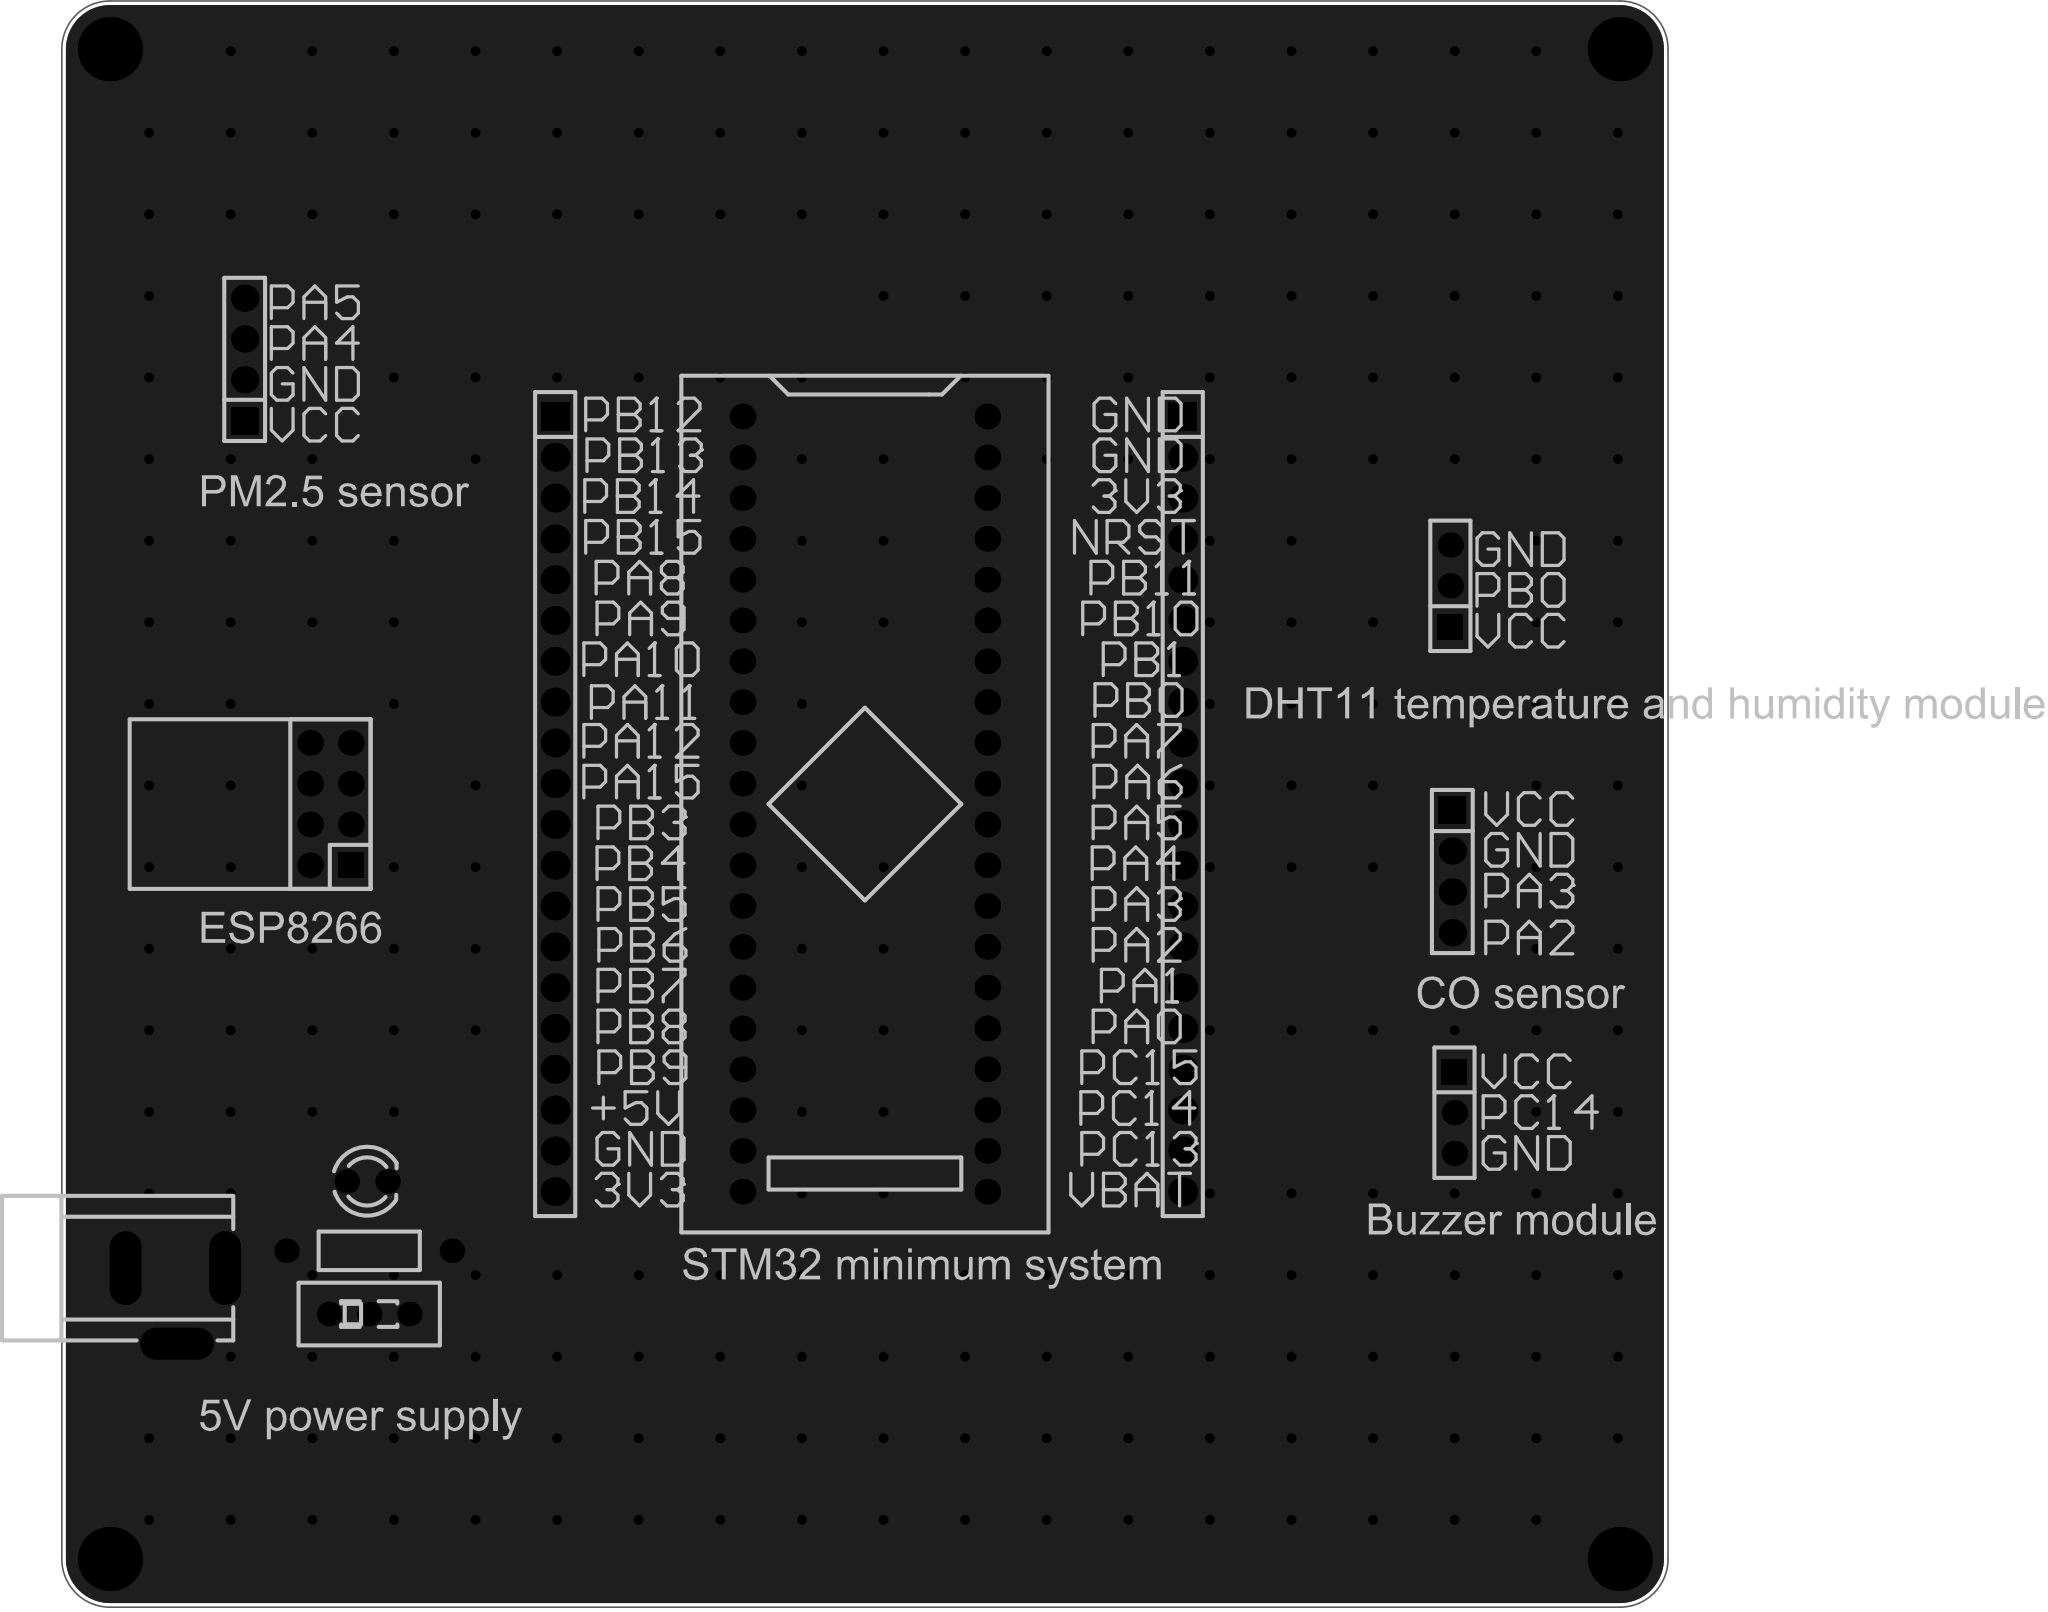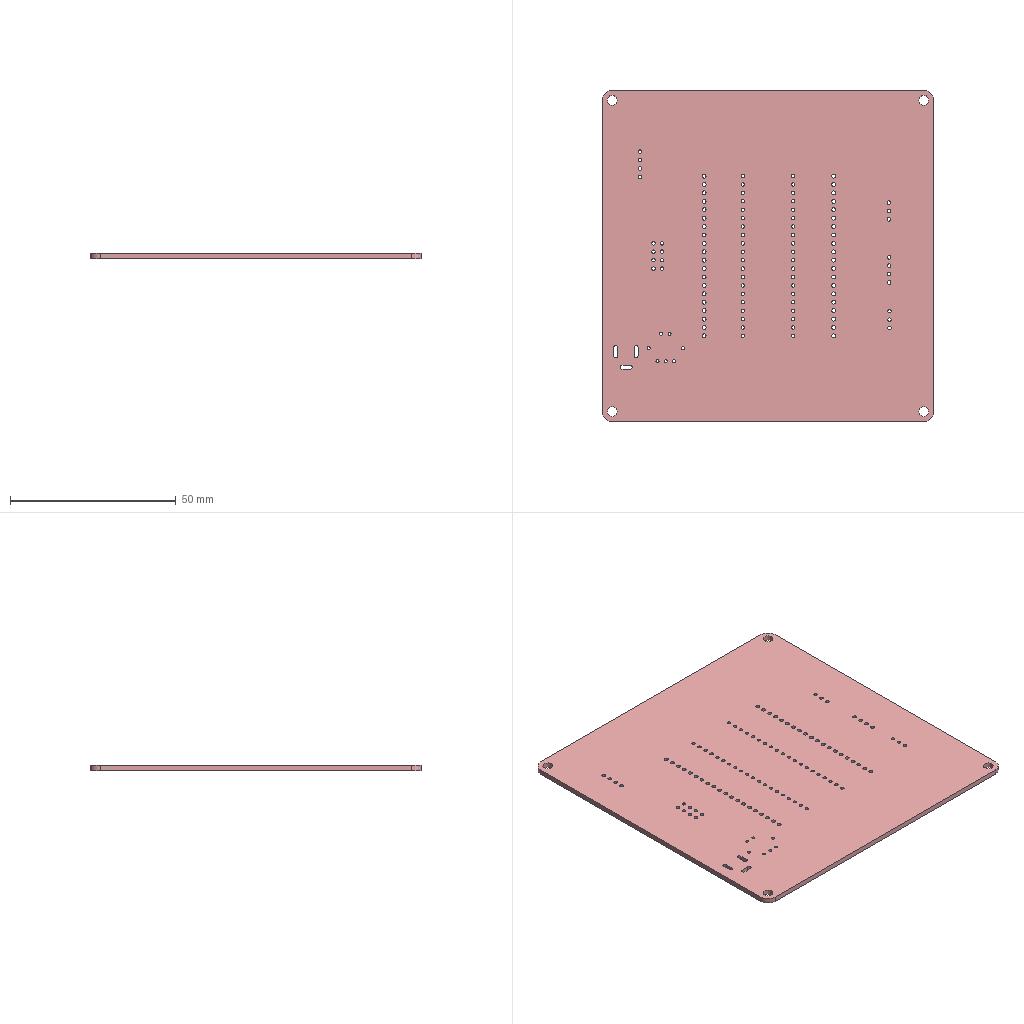Circuit board layout | Altium Designer | box 100 x 100 x 1.6 mm
Layer stack:
# Altium Designer layer stack of  (unit mm; dielectric type: 0 none, 1 core, 2 prepreg, 3 surface material)
index,name,kind,layer,copper_thickness_mm,dielectric_type,dielectric_thickness_mm,dielectric_material,dielectric_constant
0,Top Paste Mask Layer,other,,,,,,
1,Top Silkscreen Layer,other,,,,,,
2,Top Solder Mask Layer,dielectric,,,3,0.01,,3.3
3,Top Layer,copper,Top Layer,0.035,,,,
4,Dielectric1,dielectric,,,3,1.51,FR4,4.5
5,Bottom Layer,copper,Bottom Layer,0.035,,,,
6,Bottom Solder Mask Layer,dielectric,,,3,0.01,,3.3
7,Bottom Silkscreen Layer,other,,,,,,
8,Bottom Paste Mask Layer,other,,,,,,
# drill layer pairs: low layer,high layer
drill_pair,Top Layer,Bottom Layer
Part placement:
Designator,Comment,Layer,Footprint,Center-X(mm),Center-Y(mm),Rotation
U1,STM32F103C8T6-Card,TopLayer,CONN-TH_L53.3-W22.9_STM32F103C8T6-CARD,130.556,128.905,270
DC1,DC005,TopLayer,DC-IN-TH_DC005,87.63,97.663,0
H23,,TopLayer,HDR-TH_4P-P2.54-V-M,167.125,124.707,270
H24,,TopLayer,HDR-TH_4P-P2.54-V-M,91.941,156.591,90
H15,,TopLayer,HDR-TH_3P-P2.54-V-F,167.005,142.494,90
H16,,TopLayer,HDR-TH_8P-P2.54-V-F-R2-C4-S2.54-1,97.282,128.905,90
H1,,TopLayer,HDR-TH_20P-P2.54-V-F,111.273,128.905,270
H2,,TopLayer,HDR-TH_20P-P2.54-V-F,150.344,128.905,270
H18,,TopLayer,HDR-TH_3P-P2.54-V-F,167.259,109.692,270
LED1,,TopLayer,LED_TH-3mm,99.568,105.41,0
R1,330,TopLayer,Res_1/4W,99.695,101.092,180
SW1,Switch,TopLayer,SW-TH_SS-12D01-GX,99.695,97.155,0
Pad and via stacks:
# Altium Designer via and pad stacks of  (unit mm). Each distinct definition once, with the count of objects using it.
# via: kind,start_layer,end_layer,hole_mm,diameter_mm,mode(0 simple;1 top-mid-bottom;2 full stack),diameter_per_layer,count,example_net
# pad: kind,layer,hole_mm,hole_type(0 round;1 square;2 slot),plating,top_size,top_shape(1 round;2 rect;3 octagon;9 rounded rect),mid_size,bottom_size,mode,footprint,size_per_layer,count,example
pad,Multi-Layer,3,0,plated,4x4,1,4x4,4x4,0,,,4,1
pad,Multi-Layer,1,0,plated,1.6x1.6,1,1.6x1.6,1.6x1.6,0,CONN-TH_L53.3-W22.9_STM32F103C8T6-CARD,,40,U1.1
pad,Multi-Layer,1.2,2,plated,2x4.6,1,2x4.6,2x4.6,0,DC-IN-TH_DC005,,2,DC1.1
pad,Multi-Layer,1.2,2,plated,4.6x2,1,4.6x2,4.6x2,0,DC-IN-TH_DC005,,1,DC1.3
pad,Multi-Layer,1.1,0,plated,1.7x1.7,2,1.7x1.7,1.7x1.7,0,HDR-TH_4P-P2.54-V-M,,2,H23.1
pad,Multi-Layer,1.1,0,plated,1.7x1.7,1,1.7x1.7,1.7x1.7,0,HDR-TH_4P-P2.54-V-M,,6,H23.2
pad,Multi-Layer,1.02,0,plated,1.575x1.575,1,1.575x1.575,1.575x1.575,0,HDR-TH_3P-P2.54-V-F,,4,H15.3
pad,Multi-Layer,1.02,0,plated,1.575x1.575,2,1.575x1.575,1.575x1.575,0,HDR-TH_3P-P2.54-V-F,,2,H15.1
pad,Multi-Layer,1.1,0,plated,1.6x1.6,2,1.6x1.6,1.6x1.6,0,HDR-TH_8P-P2.54-V-F-R2-C4-S2.54-1,,1,H16.1
pad,Multi-Layer,1.1,0,plated,1.6x1.6,1,1.6x1.6,1.6x1.6,0,HDR-TH_8P-P2.54-V-F-R2-C4-S2.54-1,,7,H16.2
pad,Multi-Layer,1.2,0,plated,1.8x1.8,2,1.8x1.8,1.8x1.8,0,HDR-TH_20P-P2.54-V-F,,2,H1.1
pad,Multi-Layer,1.2,0,plated,1.8x1.8,1,1.8x1.8,1.8x1.8,0,HDR-TH_20P-P2.54-V-F,,38,H1.2
pad,Multi-Layer,0.9144,0,plated,1.524x1.524,1,1.524x1.524,1.524x1.524,0,LED_TH-3mm,,2,LED1.1
pad,Multi-Layer,1,0,plated,1.524x1.524,1,1.524x1.524,1.524x1.524,0,Res_1/4W,,2,R1.1
pad,Multi-Layer,0.9144,0,plated,1.524x1.524,1,1.524x1.524,1.524x1.524,0,SW-TH_SS-12D01-GX,,3,SW1.1
via,Top Layer,Bottom Layer,0.3048,0.61,0,,258,GND
Copper pours:
name,layer,net,type(0 solid;1 hatched;2 none)
Bottom Layer-GND,Bottom Layer,GND,0
Top Layer-GND,Top Layer,GND,0